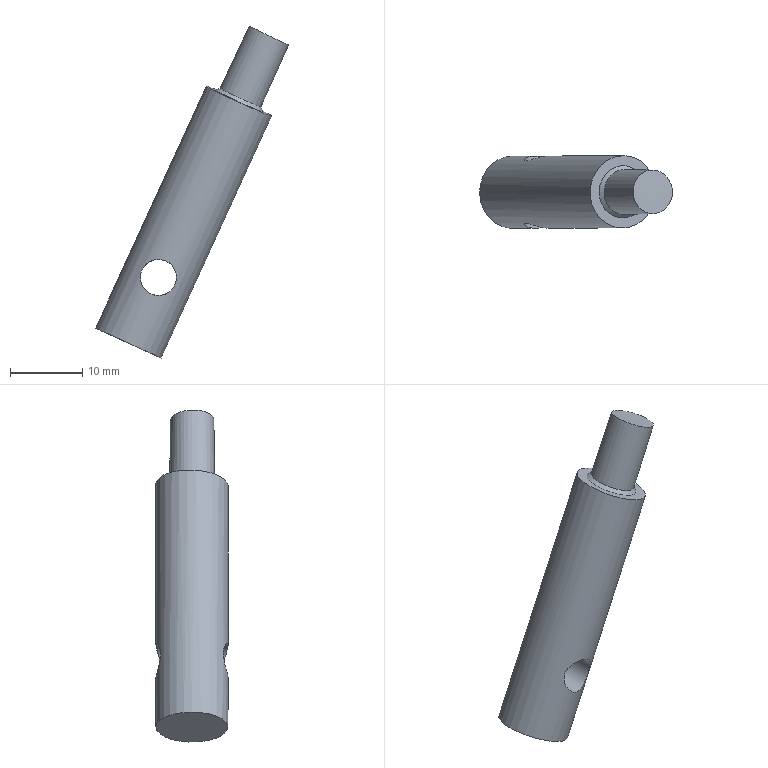Part | STEP file | solid 93 | 1 solid | 7 faces | box 26.72 x 10 x 46.022 mm | volume 3002 mm3 | cylinder 2 | plane 2 | spline 2 | cone 1 | commonest cylinder face diameters 5 x1 10 x1